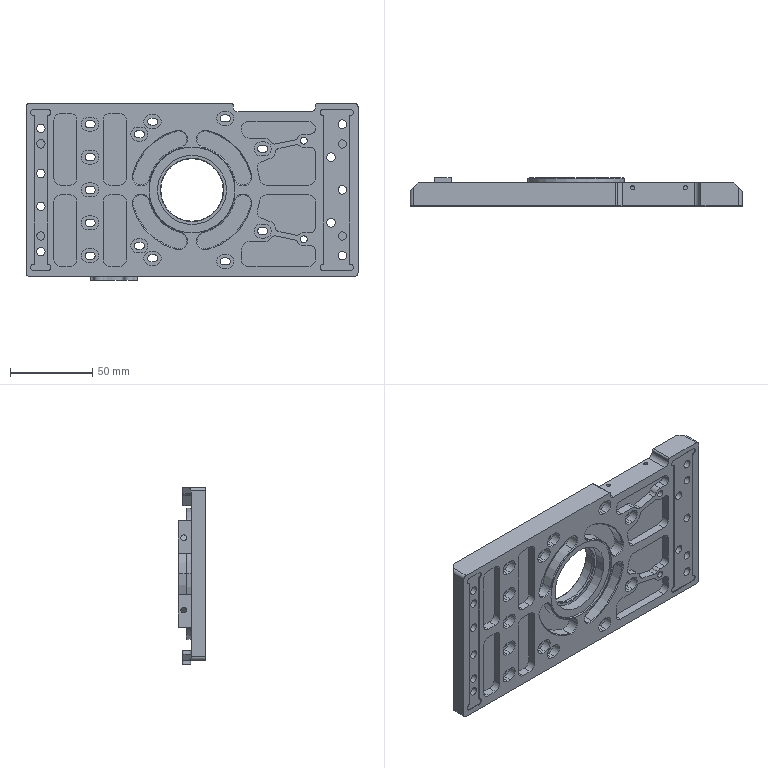NC program | Mastercam | posted with a generic post | part box 202 x 17 x 107.5 mm
Lines 1 to 36 of 36425:
%
:0001()
(MATERIAL - ALUMINUM MM - 2024)
(T24|100 FEM |H24)
(T10|10 FEM |H10|XY STOCK TO LEAVE - .15|Z STOCK TO LEAVE - 0.)
(T6|6 FEM |H6|XY STOCK TO LEAVE - .1|Z STOCK TO LEAVE - 0.)
(T11|10 FEM |H11)
(T8|8 FEM |H8|XY STOCK TO LEAVE - .1|Z STOCK TO LEAVE - .1)
(T5|5 FEM |H5|XY STOCK TO LEAVE - .07|Z STOCK TO LEAVE - .07)
(T4|4 FEM |H4|XY STOCK TO LEAVE - -.01|Z STOCK TO LEAVE - 0.)
(T3|3 FEM |H3|XY STOCK TO LEAVE - .1|Z STOCK TO LEAVE - .1)
(T7|4 CHM |H7)
(T9|8 BNOS |H9)
(T15|4 BM/BNOS |H15)
(T1|3.3 DR |H1)
N100 G21
N102 G0 G17 G40 G80 G90 G94 G98
N104 G0 G28 G91 Z0.
N106 G0 G28 X0. Y0.
(100 FEM |TOOL - 24|DIA. OFF. - 24|LEN. - 24|TOOL DIA. - 100.)
N108 T24 M6
N110 G0 G54 G90 X-170. Y22.498 C0. B0. S4000 M3
N112 G43 H24 Z25.
N114 Z1.
N116 G1 Z0. F600.
N118 X165. F1000.
N120 G2 X187.498 Y0. J-22.498
N122 X165. Y-22.498 I-22.498
N124 G1 X-170.
N126 G0 Z25.
N128 M5
N130 G0 G28 G91 Z0.
N132 G28
N134 M01
N136 G0 G17 G40 G80 G90 G94 G98
N138 G0 G28 G91 Z0.